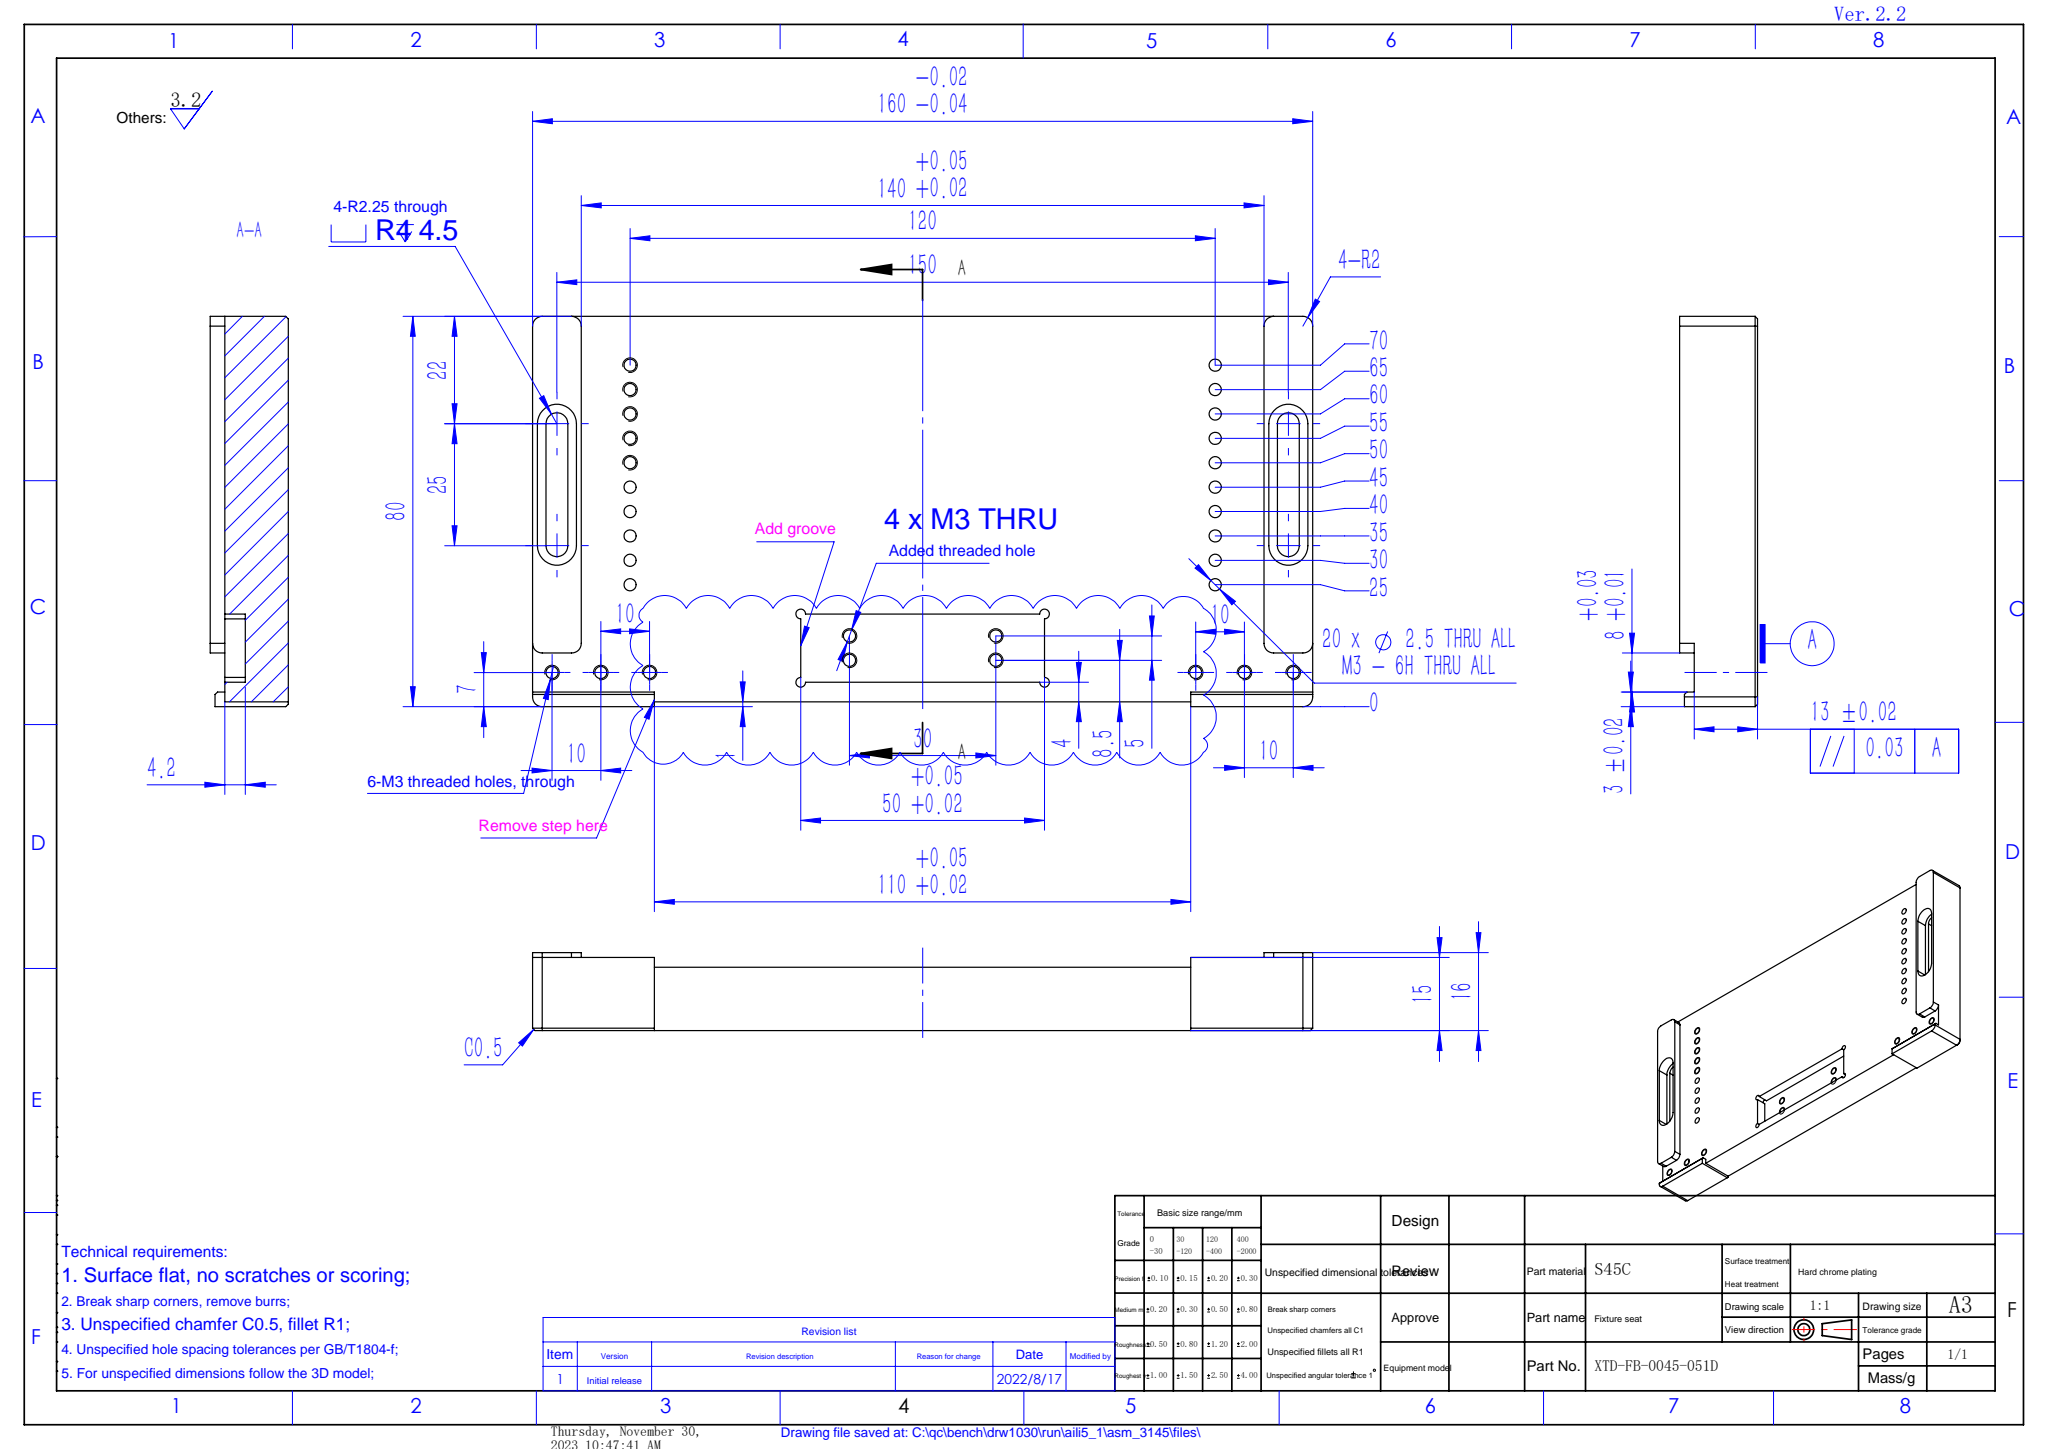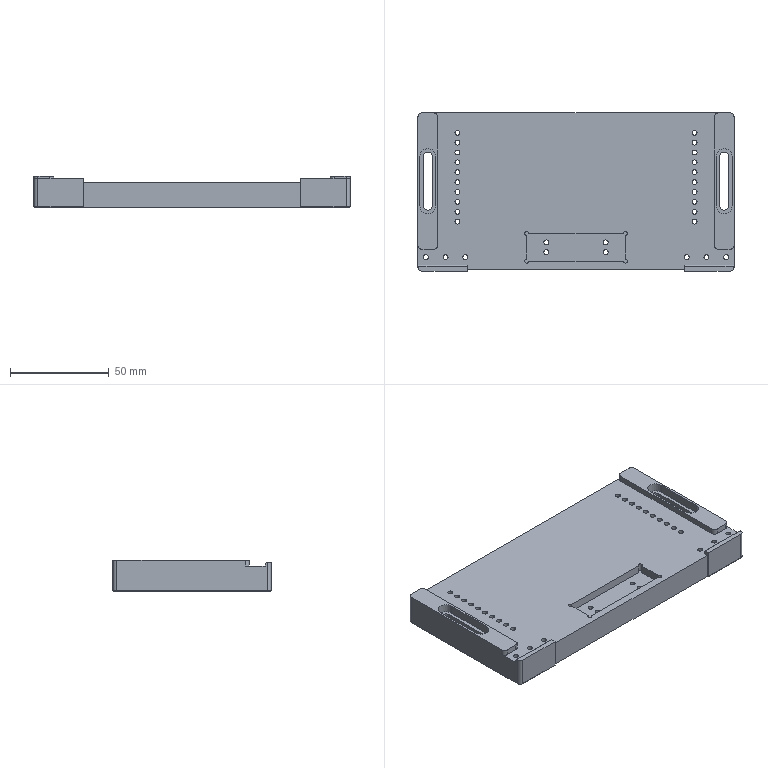Part | SolidWorks | features ICE 8, HoleWzd 5, Chamfer 4, Extrusion 1, Fillet 1, LPattern 1 | 1 solid | 130 faces | box 160 x 80 x 16 mm | volume 159297 mm3 | cylinder 84 | plane 42 | cone 4 | commonest cylinder face diameters 2.5 x60 4 x10 2 x6 4.5 x4 8 x4